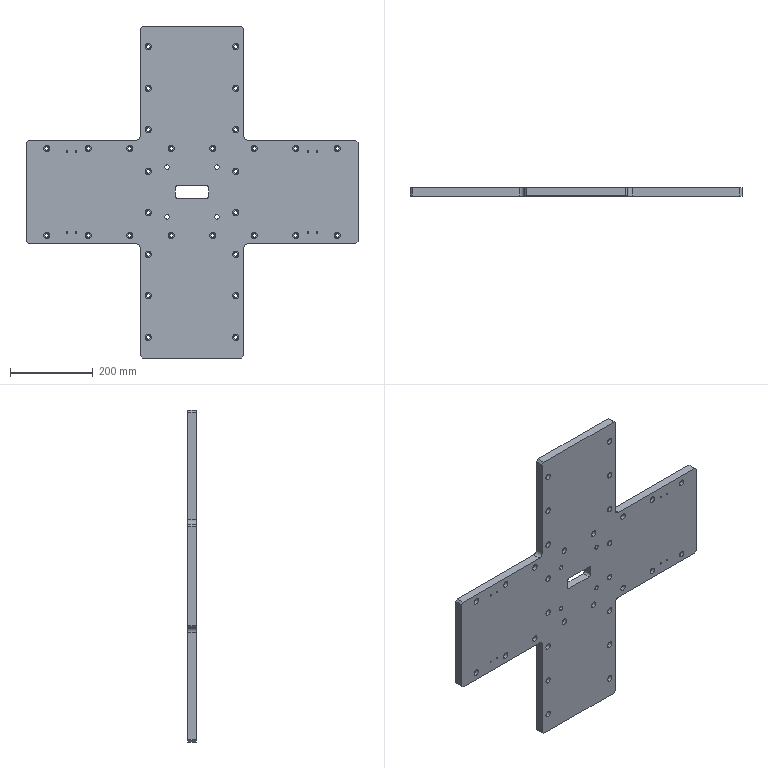Part | SolidWorks | features HoleWzd 3, Chamfer 1, Cut 1, Extrusion 1, Fillet 1 | 1 solid | 218 faces | box 800 x 20 x 800 mm | volume 6619888 mm3 | cylinder 160 | plane 58 | commonest cylinder face diameters 9 x64 15 x64 3.3 x16 11 x8 10 x4 20 x4